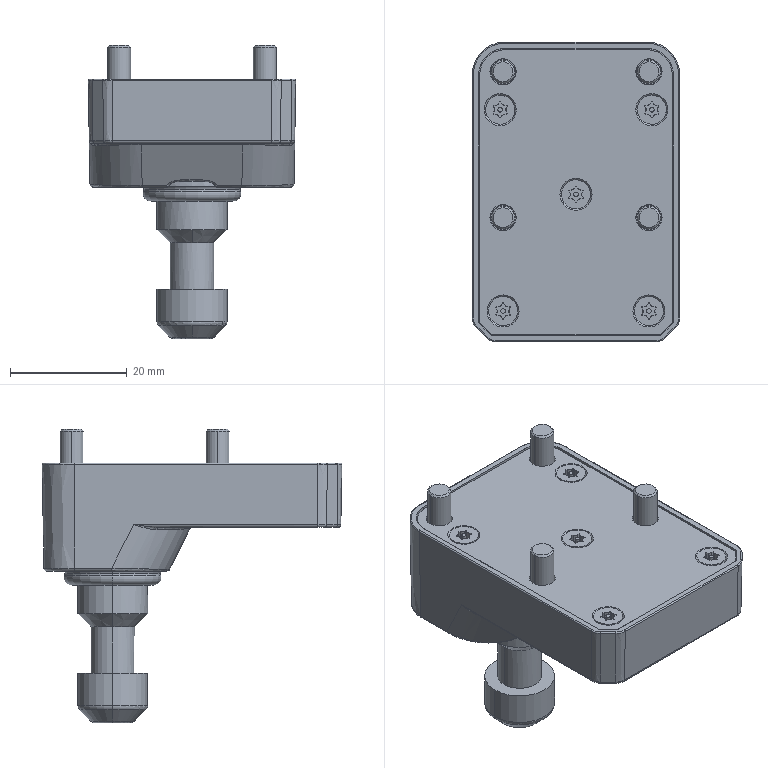Part | SolidWorks | features BaseBody 15 | 15 solids | 1119 faces | box 35.586 x 51.386 x 50.3 mm | volume 17360 mm3 | plane 403 | cone 274 | cylinder 271 | torus 87 | spline 72 | sphere 12 | commonest cylinder face diameters 1 x41 0.4 x18 7.513 x16 0.8 x14 1.8 x12 2.7 x12